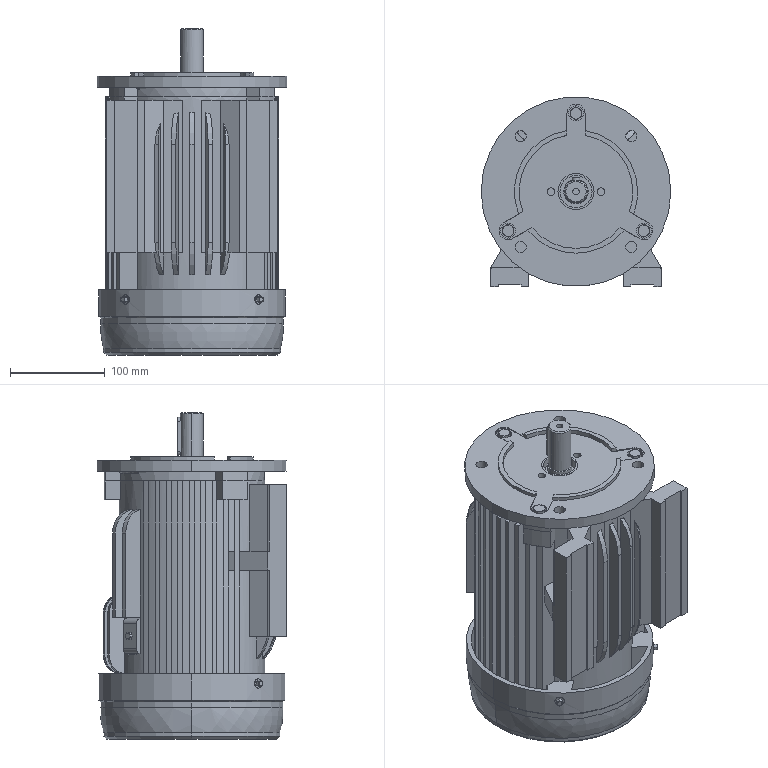Part | SolidWorks | features ICE 8, BaseBody 1 | 1 solid | 454 faces | box 200 x 200 x 344.5 mm | volume 7028641 mm3 | plane 272 | cylinder 146 | cone 30 | spline 6 | commonest cylinder face diameters 183 x19 10 x16 1 x14 40 x10 100 x10 12 x8